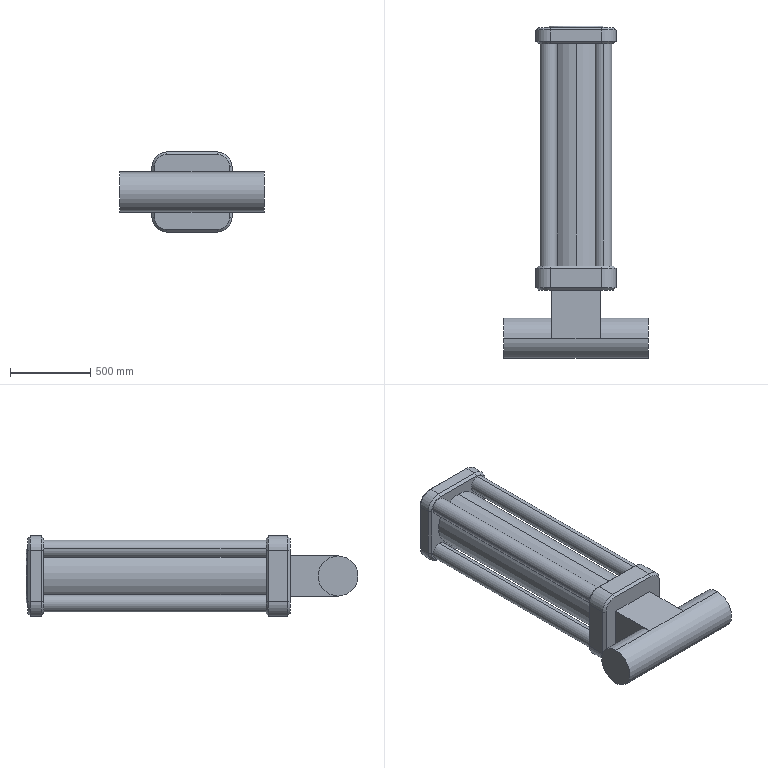Part | SolidWorks | features ICE 5, Chamfer 2, CirPattern 1, Extrusion 1, Fillet 1 | 1 solid | 77 faces | box 900 x 2075 x 500 mm | volume 199236991 mm3 | plane 36 | cylinder 23 | cone 18 | commonest cylinder face diameters 108.453 x8 180 x8 250 x3 300 x2 350 x2